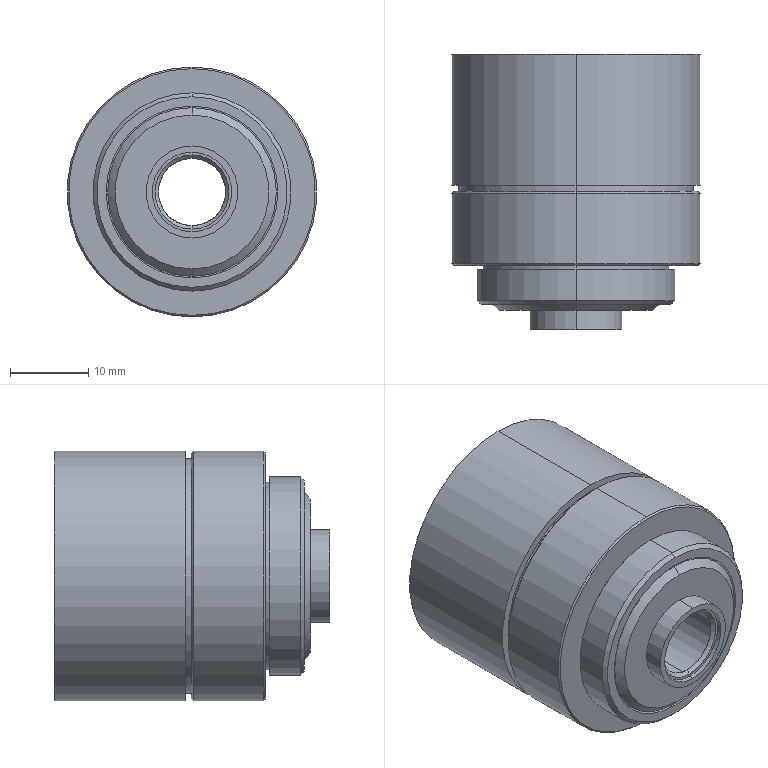Part | SolidWorks | features Revolution 1 | 2 solids | 79 faces | box 32 x 35.3 x 32 mm | volume 16584 mm3 | cylinder 44 | plane 23 | cone 12 | commonest cylinder face diameters 22 x4 24 x4 30 x4 32 x4 10 x2 10.2 x2